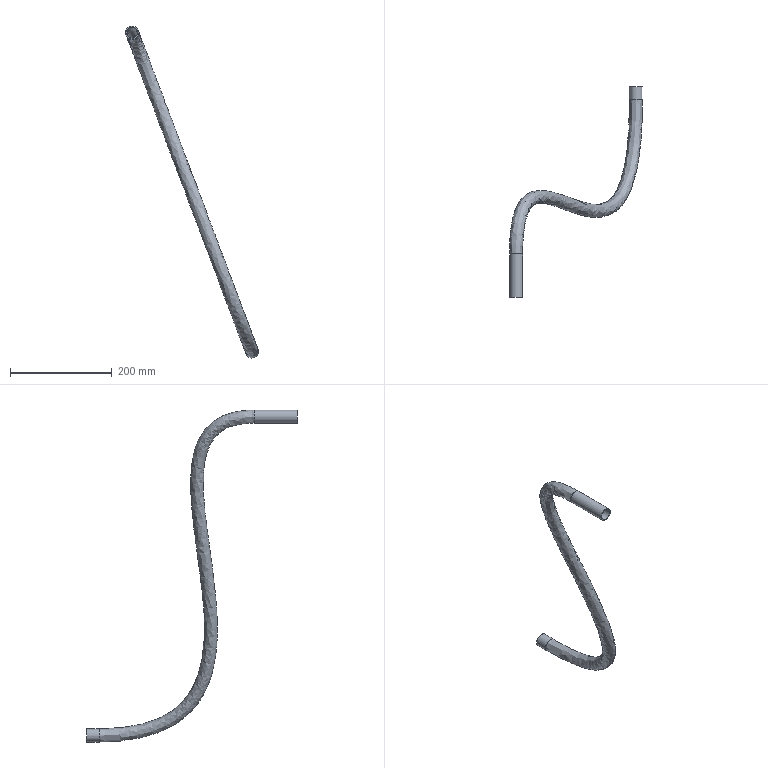Part | STEP file | Part 3^JBJ-F-0000-00 | 1 solid | 8 faces | box 261.691 x 414.992 x 653.065 mm | volume 148714 mm3 | cylinder 4 | spline 2 | plane 2 | commonest cylinder face diameters 22 x2 26 x2